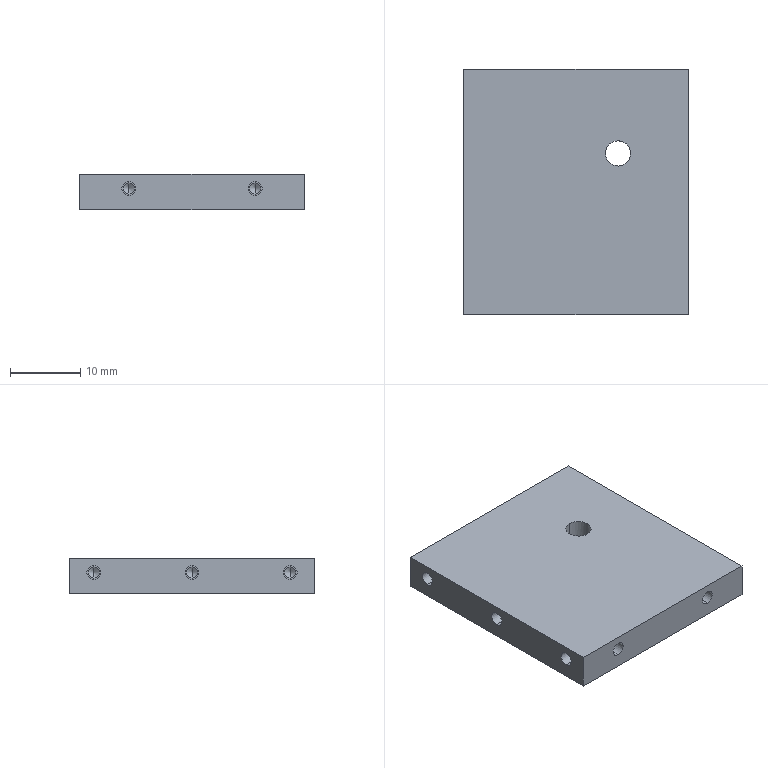Part | STEP file | ASND-0110-OPT-CO40-X-V1.0 rear cover plate | 1 solid | 108 faces | box 32 x 35 x 5 mm | volume 5286 mm3 | cylinder 58 | cone 30 | plane 20 | commonest cylinder face diameters 1.6 x20 2 x20 2.5 x8 3 x8 3.6 x2